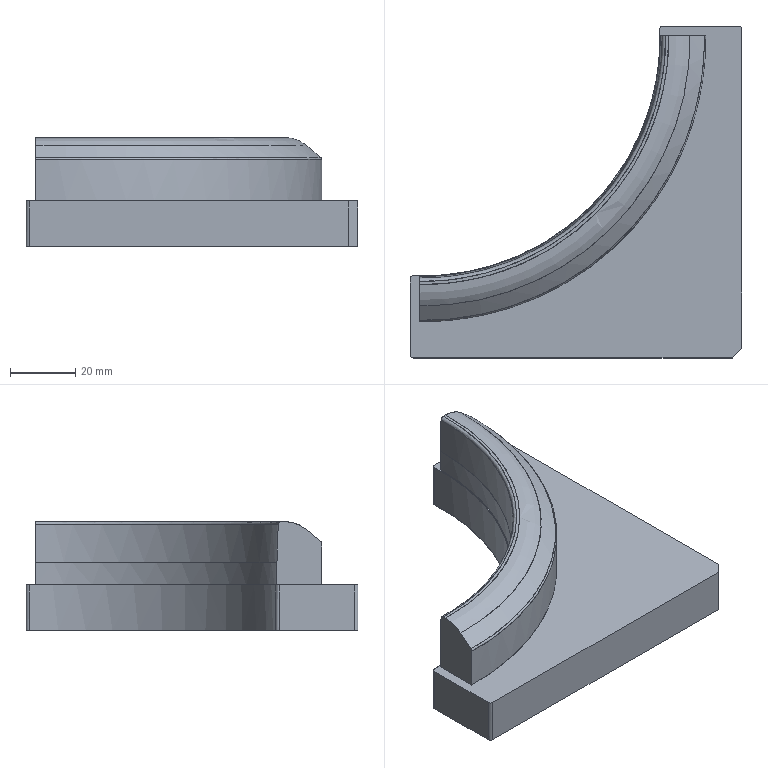NC program | PowerMill | posted with a generic post | part box 102 x 102 x 33.478 mm
Lines 26163 to 27589 of 321973:
N26260 M6
N26261 S8500 M03
N26262 G00 G90 X0.0 Y0.0
N26263 G43 Z11.798 H3
N26264
N26265 G05 P10000 R8
N26266 X-44.9733 Y-16.6515
N26267 Z0.9284
N26268 G01 Z-0.2716 F360.0
N26269 X-44.7623 Y-21.9223 F600.0
N26270 X-52.3322 Y-32.1075
N26271 X-52.0765 Y-32.4201
N26272 X-51.698 Y-32.7961
N26273 X-51.4398 Y-33.0238
N26274 X-51.2774 Y-33.1416
N26275 X-51.1104 Y-33.2689
N26276 X-50.8427 Y-33.4358
N26277 X-50.7894 Y-33.4748
N26278 X-50.4661 Y-33.6516
N26279 X-50.2251 Y-33.7596
N26280 X-50.1454 Y-33.8005
N26281 X-49.8233 Y-33.9257
N26282 X-49.497 Y-34.0292
N26283 X-49.2456 Y-34.0811
N26284 X-49.1782 Y-34.1097
N26285 X-48.8563 Y-34.167
N26286 X-48.5373 Y-34.205
N26287 X-48.2139 Y-34.2338
N26288 X-47.9403 Y-34.2383
N26289 X-38.4079 Y-21.4126
N26290 X-37.7927 Y-21.3346
N26291 X-36.8455 Y-21.201
N26292 X-36.2144 Y-21.1043
N26293 X-35.2671 Y-20.9472
N26294 X-34.636 Y-20.8355
N26295 X-33.6888 Y-20.6565
N26296 X-32.7418 Y-20.4631
N26297 X-31.5277 Y-20.1954
N26298 X-41.8701 Y-34.111
N26299 X-41.4021 Y-34.0852
N26300 X-41.2489 Y-34.0705
N26301 X-40.9258 Y-34.0486
N26302 X-40.6131 Y-34.0011
N26303 X-39.9854 Y-33.9497
N26304 X-39.3505 Y-33.912
N26305 X-38.4006 Y-33.8202
N26306 X-37.9379 Y-33.7685
N26307 X-37.7675 Y-33.7437
N26308 X-37.451 Y-33.7138
N26309 X-36.8169 Y-33.6351
N26310 X-36.5021 Y-33.5904
N26311 X-36.1825 Y-33.5538
N26312 X-35.8626 Y-33.5014
N26313 X-35.6198 Y-33.452
N26314 X-35.3807 Y-33.4197
N26315 X-23.8954 Y-17.9663
N26316 X-23.5866 Y-17.858
N26317 X-22.9558 Y-17.6264
N26318 X-21.3769 Y-17.0172
N26319 X-20.1399 Y-16.5055
N26320 X-19.4029 Y-16.1898
N26321 X-18.2203 Y-15.6594
N26322 X-16.9573 Y-15.065
N26323 X-16.0414 Y-14.6114
N26324 X-15.0494 Y-14.1042
N26325 X-28.4407 Y-32.1221
N26326 X-28.2757 Y-32.0895
N26327 X-27.9566 Y-32.0117
N26328 X-27.6359 Y-31.9409
N26329 X-27.3579 Y-31.8612
N26330 X-27.3099 Y-31.8361
N26331 X-26.6913 Y-31.6679
N26332 X-26.3741 Y-31.604
N26333 X-26.0579 Y-31.5255
N26334 X-25.4226 Y-31.3594
N26335 X-24.4741 Y-31.0918
N26336 X-23.8756 Y-30.9169
N26337 X-23.8357 Y-30.9007
N26338 X-23.209 Y-30.7123
N26339 X-22.8875 Y-30.6234
N26340 X-22.5661 Y-30.5105
N26341 X-22.3787 Y-30.4327
N26342 X-22.2613 Y-30.398
N26343 X-21.8412 Y-30.287
N26344 X-21.6225 Y-30.2161
N26345 X-21.3074 Y-30.1042
N26346 X-20.8541 Y-29.9544
N26347 X-3.3016 Y-6.3377
N26348 X-2.62 Y-5.7722
N26349 X-1.8042 Y-5.075
N26350 X-1.1729 Y-4.5225
N26351 X-0.4587 Y-3.8781
N26352 X0.0896 Y-3.3689
N26353 X0.8843 Y-2.6153
N26354 X1.8467 Y-1.6681
N26355 X2.468 Y-1.0369
N26356 X3.3707 Y-0.0897
N26357 X3.9523 Y0.5416
N26358 X4.5095 Y1.1591
N26359 X5.0782 Y1.8044
N26360 X5.6188 Y2.4358
N26361 X6.0877 Y2.9945
N26362 X6.9149 Y4.0142
N26363 X7.3505 Y4.569
N26364 X7.9821 Y5.3896
N26365 X8.3701 Y5.9082
N26366 X8.9291 Y6.6715
N26367 X9.5104 Y7.4868
N26368 X9.9448 Y8.118
N26369 X10.5075 Y8.9534
N26370 X10.9916 Y9.6965
N26371 X11.591 Y10.6435
N26372 X12.3554 Y11.9065
N26373 X12.7172 Y12.5268
N26374 X13.2609 Y13.4849
N26375 X13.6229 Y14.147
N26376 X13.98 Y14.8118
N26377 X14.4363 Y15.6945
N26378 X14.9271 Y16.6765
N26379 X15.3661 Y17.5889
N26380 X15.6599 Y18.22
N26381 X16.0871 Y19.167
N26382 X16.6704 Y20.5345
N26383 X34.2205 Y44.148
N26384 X34.246 Y44.7322
N26385 X34.269 Y45.6838
N26386 X34.2668 Y45.9989
N26387 X34.2784 Y46.9517
N26388 X34.2651 Y47.2717
N26389 X34.2403 Y47.5841
N26390 X34.2388 Y47.9011
N26391 X34.2298 Y48.218
N26392 X34.2109 Y48.5411
N26393 X34.169 Y48.8654
N26394 X34.1019 Y49.1798
N26395 X34.0826 Y49.2883
N26396 X34.0266 Y49.5072
N26397 X33.9236 Y49.8292
N26398 X33.7978 Y50.1516
N26399 X33.6465 Y50.4729
N26400 X33.465 Y50.8042
N26401 X33.4352 Y50.841
N26402 X33.3375 Y51.0
N26403 X20.7223 Y34.0264
N26404 X20.9252 Y35.1255
N26405 X21.0671 Y35.9852
N26406 X21.2025 Y36.8459
N26407 X21.4191 Y38.4243
N26408 X21.5307 Y39.3712
N26409 X21.597 Y40.0023
N26410 X21.7145 Y41.2656
N26411 X21.7648 Y41.8964
N26412 X21.8074 Y42.5278
N26413 X21.8678 Y43.6077
N26414 X29.1911 Y53.4612
N26415 X29.2555 Y53.4571
N26416 X29.5776 Y53.418
N26417 X29.8517 Y53.3677
N26418 X30.2209 Y53.2783
N26419 X30.5437 Y53.1803
N26420 X30.8973 Y53.0451
N26421 X31.1888 Y52.9092
N26422 X31.4956 Y52.7392
N26423 X31.5378 Y52.7225
N26424 X31.8298 Y52.5358
N26425 X32.023 Y52.4011
N26426 X32.1529 Y52.3001
N26427 X32.419 Y52.0775
N26428 X32.7487 Y51.7555
N26429 X33.0301 Y51.4319
N26430 X33.1176 Y51.3096
N26431 X33.2699 Y51.1099
N26432 X33.4352 Y50.841
N26433 X33.475 Y50.7891
N26434 X33.6491 Y50.4678
N26435 X33.8005 Y50.1454
N26436 X33.9257 Y49.8233
N26437 X34.0282 Y49.5015
N26438 X34.0842 Y49.2809
N26439 X34.1019 Y49.1798
N26440 X34.1704 Y48.8572
N26441 X34.2116 Y48.5341
N26442 X34.2298 Y48.218
N26443 X34.2388 Y47.9011
N26444 X34.2403 Y47.5841
N26445 X34.2653 Y47.2679
N26446 X34.2784 Y46.9464
N26447 X34.2668 Y45.9989
N26448 X34.269 Y45.6806
N26449 X34.246 Y44.7322
N26450 X34.2045 Y43.7833
N26451 X34.1998 Y43.4615
N26452 X34.146 Y42.8315
N26453 X34.1334 Y42.5193
N26454 X34.1318 Y42.2003
N26455 X34.1156 Y41.8842
N26456 X33.9998 Y40.3013
N26457 X33.884 Y39.0283
N26458 X33.834 Y38.7142
N26459 X33.7691 Y38.1527
N26460 X33.7134 Y37.4522
N26461 X33.6779 Y37.1326
N26462 X33.6317 Y36.8173
N26463 X33.4665 Y35.5506
N26464 X33.4164 Y35.2364
N26465 X33.3862 Y34.9854
N26466 X-12.3068 Y-26.4943
N26467 X-12.1313 Y-26.4169
N26468 X-11.1785 Y-25.9602
N26469 X-10.8567 Y-25.7993
N26470 X-10.5425 Y-25.6165
N26471 X-10.2304 Y-25.4527
N26472 X-9.9082 Y-25.3022
N26473 X-9.7749 Y-25.2244
N26474 X-9.594 Y-25.1569
N26475 X-9.2809 Y-24.9837
N26476 X-9.1142 Y-24.9058
N26477 X-8.5155 Y-24.5878
N26478 X-8.3296 Y-24.4801
N26479 X-8.0063 Y-24.3103
N26480 X-7.9479 Y-24.2714
N26481 X-7.6964 Y-24.1413
N26482 X-7.0646 Y-23.7841
N26483 X-6.7964 Y-23.6369
N26484 X-6.43 Y-23.401
N26485 X-6.2839 Y-23.3218
N26486 X-6.1155 Y-23.2176
N26487 X-5.7975 Y-23.0531
N26488 X-5.1705 Y-22.677
N26489 X-5.1567 Y-22.664
N26490 X-4.8483 Y-22.4913
N26491 X-4.5308 Y-22.2984
N26492 X-4.0848 Y-22.0176
N26493 X-3.627 Y-21.7347
N26494 X-3.5781 Y-21.6963
N26495 X-3.1414 Y-21.4219
N26496 X-2.6877 Y-21.1066
N26497 X-2.2098 Y-20.7927
N26498 X-2.0071 Y-20.6761
N26499 X30.7888 Y23.4504
N26500 G00 Z11.798
N26501 G05 P0
N26502 (---------------)
N26503 ( END TOOLPATH : 精公基准台01-平坦面平行-D10 )
N26504 (---------------)
N26505 ( START TOOLPATH : 精公基准台01-基准面偏置-D10 )
N26506 (---------------)
N26507 G00 X0.0 Y0.0 Z9.7984
N26508 G05 P10000 R8
N26509 X-47.5023 Y-15.0387
N26510 Z-18.48
N26511 G01 Z-19.68 F360.0
N26512 X-47.5975 Y-20.3128 F600.0
N26513 X-47.6004 Y-20.7252
N26514 G03 X-45.617 Y-20.7134 I0.5299 J77.1533
N26515 G01 X-44.4837 Y-20.6813
N26516 G03 X-42.217 Y-20.559 I-3.0409 J77.4268
N26517 G03 X-37.9216 Y-20.1168 I-4.9741 J69.4072
N26518 G03 X-34.425 Y-19.5501 I-9.5294 J69.8717
N26519 G01 X-33.7169 Y-19.4121
N26520 G03 X-29.7502 Y-18.4932 I-13.2081 J66.0374
N26521 G01 X-29.1836 Y-18.3432
N26522 G03 X-26.9169 Y-17.6816 I-20.7852 J75.4278
N26523 G03 X-22.5249 Y-16.1501 I-20.2295 J65.0766
N26524 G01 X-21.8168 Y-15.8715
N26525 X-20.6835 Y-15.4061
N26526 X-19.7784 Y-15.0168
N26527 G03 X-17.8501 Y-14.1333 I-28.5878 J64.9414
N26528 G03 X-16.1974 Y-13.3168 I-27.8477 J58.4463
N26529 G01 X-15.5835 Y-13.0008
N26530 G03 X-13.8834 Y-12.0791 I-36.156 J68.7183
N26531 G03 X-11.6168 Y-10.7499 I-34.8659 J62.052
N26532 G03 X-7.782 Y-8.2167 I-35.5326 J57.959
N26533 G01 X-7.6501 Y-8.1224
N26534 G03 X-5.3834 Y-6.4326 I-38.1634 J53.5581
N26535 G01 X-4.7716 Y-5.95
N26536 X-4.1728 Y-5.4673
N26537 X-3.3881 Y-4.8167
N26538 X-2.7218 Y-4.25
N26539 X-2.0749 Y-3.6834
N26540 G03 X-0.2269 Y-1.9833 I-51.4771 J57.8141
N26541 G01 X0.3589 Y-1.4167
N26542 X0.89 Y-0.89
N26543 X1.4167 Y-0.3589
N26544 X2.037 Y0.2833
N26545 X2.5694 Y0.85
N26546 X3.1167 Y1.4452
N26547 X3.6834 Y2.0749
N26548 X4.25 Y2.7218
N26549 G03 X5.95 Y4.7716 I-53.5505 J46.1433
N26550 G01 X6.4334 Y5.3834
N26551 G03 X7.7148 Y7.0834 I-57.1547 J44.4129
N26552 G01 X8.1214 Y7.6484
N26553 X8.5233 Y8.2167
N26554 G03 X9.9167 Y10.293 I-55.0628 J38.4589
N26555 G01 X10.3371 Y10.9525
N26556 X10.7499 Y11.6168
N26557 G03 X11.6168 Y13.0733 I-58.4313 J35.763
N26558 G03 X12.6995 Y15.0168 I-55.8056 J32.362
N26559 G01 X13.0008 Y15.5835
N26560 X13.5802 Y16.7168
N26561 G03 X14.4501 Y18.5233 I-63.9469 J31.906
N26562 G03 X15.7803 Y21.5933 I-61.0333 J28.2679
N26563 G01 X15.8715 Y21.8168
N26564 G03 X19.6287 Y34.8503 I-62.9275 J25.1989
N26565 G03 X20.0836 Y37.6836 I-68.3408 J12.4251
N26566 G01 X20.1175 Y37.9257
N26567 G03 X20.559 Y42.217 I-69.2604 J9.2932
N26568 G03 X20.7136 Y45.617 I-71.153 J4.9404
N26569 G03 X20.7228 Y47.8837 I-79.9998 J1.4556
N26570 G01 X20.7248 Y48.167
N26571 X20.741 Y48.4504
N26572 X20.7726 Y48.7337
N26573 X20.8193 Y49.017
N26574 X20.8817 Y49.3004
N26575 X20.9607 Y49.5837
N26576 X21.0566 Y49.867
N26577 X21.1707 Y50.1504
N26578 X21.2502 Y50.3239
N26579 X21.3493 Y50.5205
N26580 X21.4588 Y50.717
N26581 X21.6262 Y50.9848
N26582 X21.8406 Y51.2837
N26583 X22.0749 Y51.5671
N26584 X22.3835 Y51.8877
N26585 X22.6668 Y52.1402
N26586 X22.9615 Y52.3684
N26587 X23.2738 Y52.5767
N26588 X23.5168 Y52.7181
N26589 X23.7963 Y52.8607
N26590 X24.0835 Y52.9871
N26591 X24.3669 Y53.0928
N26592 X24.6502 Y53.1805
N26593 X24.9335 Y53.2515
N26594 X25.2169 Y53.3066
N26595 X25.5002 Y53.3464
N26596 X25.7835 Y53.3706
N26597 X26.0669 Y53.38
N26598 X39.9503 Y53.3789
N26599 X40.2336 Y53.3657
N26600 X40.517 Y53.3371
N26601 X40.8003 Y53.2932
N26602 X41.0836 Y53.2336
N26603 X41.367 Y53.1582
N26604 X41.6503 Y53.0654
N26605 X41.8636 Y52.9837
N26606 X42.217 Y52.8252
N26607 X42.5003 Y52.6746
N26608 X42.7837 Y52.5015
N26609 X42.9087 Y52.4171
N26610 X43.1295 Y52.255
N26611 X43.3503 Y52.0745
N26612 X43.5947 Y51.8504
N26613 X43.7631 Y51.6787
N26614 X43.917 Y51.507
N26615 X44.0988 Y51.2837
N26616 X44.3029 Y51.0004
N26617 X44.4837 Y50.7118
N26618 X44.6366 Y50.4311
N26619 X44.7687 Y50.1504
N26620 X44.8828 Y49.867
N26621 X44.9787 Y49.5837
N26622 X45.0503 Y49.3292
N26623 X45.1201 Y49.017
N26624 X45.1668 Y48.7337
N26625 X45.1984 Y48.4504
N26626 X45.2149 Y48.167
N26627 G02 X34.7155 Y4.25 I-92.1999 J-1.171
N26628 G02 X26.3502 Y-8.8999 I-81.6775 J42.7234
N26629 G01 X25.7873 Y-9.6312
N26630 X25.2169 Y-10.3567
N26631 X24.6502 Y-11.0628
N26632 G02 X18.9835 Y-17.4301 I-71.6609 J58.0708
N26633 G01 X18.1987 Y-18.2234
N26634 X31.7795 Y-31.8074
N26635 G02 X28.1412 Y-35.2825 I-77.9894 J78.008
N26636 G01 X27.3171 Y-36.0344
N26637 G03 X27.7283 Y-37.0998 I0.413 J-0.4527
N26638 G01 X35.7571 Y-37.1234
N26639 G03 X37.0941 Y-35.7868 I0.0039 J1.3331
N26640 G01 X37.0728 Y-27.7575
N26641 G03 X36.0076 Y-27.3461 I-0.6127 J-0.0016
N26642 G01 X35.2554 Y-28.1699
N26643 G02 X31.7795 Y-31.8074 I-81.4601 J74.3653
N26644 G01 X28.3843 Y-28.4114
N26645 G02 X14.3498 Y-40.2097 I-75.2562 J75.2741
N26646 G01 X13.4495 Y-40.8427
N26647 G03 X13.7703 Y-41.8622 I0.3225 J-0.4587
N26648 G01 X40.5758 Y-41.9435
N26649 G03 X41.9128 Y-40.6068 I0.004 J1.333
N26650 G01 X41.8392 Y-13.8045
N26651 G03 X40.8193 Y-13.4838 I-0.5608 J-0.0016
N26652 G01 X40.2524 Y-14.2915
N26653 G02 X37.7473 Y-17.7076 I-83.6931 J58.7486
N26654 G01 X37.6404 Y-17.8471
N26655 G02 X28.3843 Y-28.4114 I-84.5123 J64.7098
N26656 G01 X24.9893 Y-25.0156
N26657 G02 X-3.9856 Y-45.2937 I-71.9642 J71.9878
N26658 G01 X-4.7619 Y-45.6554
N26659 G03 X-4.5518 Y-46.6107 I0.2116 J-0.4542
N26660 G01 X45.078 Y-46.7627
N26661 G03 X45.9755 Y-46.4189 I0.004 J1.3329
N26662 G01 X46.2913 Y-46.1336
N26663 G03 X46.7308 Y-45.1408 I-0.8934 J0.9891
N26664 G01 X46.5929 Y4.5101
N26665 G03 X45.638 Y4.7213 I-0.5011 J-0.0014
N26666 G01 X45.1992 Y3.7844
N26667 G02 X33.8841 Y-14.8574 I-92.0187 J43.0981
N26668 G01 X33.87 Y-14.8758
N26669 G02 X24.9893 Y-25.0156 I-80.8445 J61.8477
N26670 G01 X21.5941 Y-21.6196
N26671 G03 X25.8575 Y-17.0746 I-68.5669 J68.5898
N26672 G01 X25.8637 Y-17.0675
N26673 G03 X42.4111 Y9.3268 I-72.8258 J64.041
N26674 G01 X42.4199 Y9.3476
N26675 G03 X50.0206 Y47.5866 I-89.341 J37.6331
N26676 G01 X50.0168 Y48.2056
N26677 X49.9788 Y48.8989
N26678 X49.7641 Y50.8652
N26679 G02 X51.0203 Y51.1091 I0.6381 J0.0705
N26680 G01 X51.2249 Y50.3794
N26681 G02 X51.27 Y50.0553 I-1.1676 J-0.3275
N26682 G01 X51.5416 Y-47.059
N26683 G02 X51.4164 Y-47.7613 I-2.0 J-0.0056
N26684 G01 X51.1701 Y-48.424
N26685 G02 X50.6359 Y-49.2116 I-1.8748 J0.6966
N26686 G01 X48.8574 Y-50.818
N26687 G02 X48.3764 Y-51.1397 I-1.3406 J1.4843
N26688 G01 X47.8717 Y-51.3799
N26689 G02 X47.006 Y-51.5741 I-0.8595 J1.8057
N26690 G01 X-50.0228 Y-51.2749
N26691 G02 X-50.3071 Y-51.2402 I0.0037 J1.2124
N26692 G01 X-51.0889 Y-51.0491
N26693 G02 X-50.8523 Y-49.7687 I0.1548 J0.6335
N26694 G01 X-48.1072 Y-50.1157
N26695 G03 X-39.5098 Y-50.0051 I3.9023 J30.8698
N26696 G01 X-32.3529 Y-48.9127
N26697 G03 X-9.6671 Y-42.5525 I-14.6218 J95.7927
N26698 G01 X-9.6345 Y-42.5389
N26699 G03 X21.5941 Y-21.6196 I-37.3404 J89.5112
N26700 G01 X18.1987 Y-18.2234
N26701 X17.2835 Y-19.1263
N26702 G02 X11.0628 Y-24.6502 I-64.2585 J66.0987
N26703 G01 X10.3567 Y-25.2169
N26704 G02 X-11.0652 Y-37.9335 I-57.3531 J72.2133
N26705 G02 X-48.167 Y-45.2145 I-35.9277 J84.906
N26706 G01 X-48.4504 Y-45.1984
N26707 X-48.7337 Y-45.1668
N26708 X-49.017 Y-45.1201
N26709 X-49.3292 Y-45.0503
N26710 X-49.5837 Y-44.9787
N26711 X-49.867 Y-44.8828
N26712 X-50.1504 Y-44.7687
N26713 X-50.4311 Y-44.6366
N26714 X-50.717 Y-44.4806
N26715 X-51.0004 Y-44.3028
N26716 X-51.2837 Y-44.0988
N26717 X-51.507 Y-43.917
N26718 X-51.6787 Y-43.7631
N26719 X-51.8504 Y-43.5947
N26720 X-52.0745 Y-43.3503
N26721 X-52.255 Y-43.1295
N26722 X-52.4171 Y-42.9087
N26723 X-52.5015 Y-42.7837
N26724 X-52.6747 Y-42.5003
N26725 X-52.8252 Y-42.217
N26726 X-52.9837 Y-41.8636
N26727 X-53.0654 Y-41.6503
N26728 X-53.158 Y-41.367
N26729 X-53.2336 Y-41.0836
N26730 X-53.2931 Y-40.8003
N26731 X-53.3371 Y-40.517
N26732 X-53.3656 Y-40.2336
N26733 X-53.3789 Y-39.9503
N26734 X-53.3801 Y-26.0669
N26735 X-53.3706 Y-25.7835
N26736 X-53.3462 Y-25.5002
N26737 X-53.3066 Y-25.2169
N26738 X-53.2515 Y-24.9335
N26739 X-53.1805 Y-24.6502
N26740 X-53.0926 Y-24.3669
N26741 X-52.9871 Y-24.0835
N26742 X-52.8608 Y-23.7963
N26743 X-52.7181 Y-23.5168
N26744 X-52.5765 Y-23.2738
N26745 X-52.4171 Y-23.0307
N26746 X-52.3601 Y-22.9502
N26747 X-52.1404 Y-22.6668
N26748 X-51.8877 Y-22.3835
N26749 X-51.7307 Y-22.2256
N26750 X-51.5671 Y-22.0745
N26751 X-51.2525 Y-21.8168
N26752 X-50.9848 Y-21.6259
N26753 X-50.717 Y-21.4588
N26754 X-50.5205 Y-21.3489
N26755 X-50.3239 Y-21.2502
N26756 X-50.1504 Y-21.1707
N26757 X-49.867 Y-21.0563
N26758 X-49.5837 Y-20.9607
N26759 X-49.3004 Y-20.8818
N26760 X-49.017 Y-20.8193
N26761 X-48.7337 Y-20.7724
N26762 X-48.4504 Y-20.741
N26763 X-48.167 Y-20.7249
N26764 X-47.6004 Y-20.7252
N26765 X-47.5975 Y-20.3128
N26766 G00 Z9.7984
N26767 G05 P0
N26768 (---------------)
N26769 ( END TOOLPATH : 精公基准台01-基准面偏置-D10 )
N26770 (---------------)
N26771 ( START TOOLPATH : 精公基准台01-外形侧光-D10 )
N26772 (---------------)
N26773 G00 X0.0 Y0.0 Z10.798
N26774 G05 P10000 R8
N26775 X19.0356 Y-17.484
N26776 Z-14.65
N26777 G01 Z-19.65 F360.0
N26778 G03 X17.9751 Y-17.9238 I0.0006 J-1.5 F600.0
N26779 G02 X13.9269 Y-21.7376 I-65.048 J64.9911
N26780 G01 X12.8309 Y-22.6934
N26781 G02 X-4.162 Y-34.2515 I-59.8408 J69.7079
N26782 G01 X-5.4409 Y-34.9132
N26783 G02 X-10.3744 Y-37.2348 I-42.0489 J82.9539
N26784 G02 X-17.5 Y-39.9867 I-36.8136 J84.7221
N26785 G02 X-35.5892 Y-44.1411 I-29.5187 J87.0706
N26786 G01 X-37.0508 Y-44.3123
N26787 G02 X-48.014 Y-44.8471 I-9.9531 J91.4064
N26788 G02 X-53.01 Y-39.7973 I0.0146 J5.0108
N26789 G01 Y-26.1041
N26790 G02 X-48.0119 Y-21.0924 I5.01 J0.0017
N26791 G03 X-37.8002 Y-20.4738 I0.9669 J68.6279
N26792 G03 X21.0965 Y46.6134 I-9.2004 J67.4739
N26793 G03 X21.0924 Y48.014 I-64.7503 J0.5105
N26794 G02 X26.1056 Y53.01 I5.0101 J-0.014
N26795 G01 X37.1235
N26796 X39.7982
N26797 G02 X44.8471 Y48.0128 I0.0383 J-5.0105
N26798 G02 X34.9127 Y5.4399 I-91.8589 J-1.0104
N26799 G01 X34.2512 Y4.1613
N26800 G02 X25.2553 Y-9.7106 I-81.2829 J42.8589
N26801 G01 X24.3692 Y-10.8215
N26802 G02 X17.9751 Y-17.9238 I-71.4416 J57.8882
N26803 G03 X17.5362 Y-18.9846 I1.0611 J-1.0602
N26804 G01 X18.979 Y-17.4274
N26805 G03 X17.9185 Y-17.8672 I0.0007 J-1.5
N26806 G02 X13.8743 Y-21.6773 I-64.9908 J64.9339
N26807 G01 X12.7789 Y-22.6325
N26808 G02 X-4.1988 Y-34.1805 I-59.7888 J69.647
N26809 G01 X-5.4767 Y-34.8417
N26810 G02 X-10.4057 Y-37.1612 I-42.0158 J82.888
N26811 G02 X-17.5254 Y-39.9108 I-36.7826 J84.6494
N26812 G02 X-35.5985 Y-44.0617 I-29.4934 J86.9953
N26813 G01 X-37.0589 Y-44.2327
N26814 G02 X-48.0123 Y-44.7671 I-9.9452 J91.3293
N26815 G02 X-52.93 Y-39.7973 I0.0129 J4.9307
N26816 G01 Y-26.1056
N26817 G02 X-48.0123 Y-21.1724 I4.93 J0.0032
N26818 G03 X-34.5031 Y-20.0233 I0.9655 J68.6338
N26819 G03 X21.1765 Y46.6127 I-12.4991 J67.0243
N26820 G03 X21.1724 Y48.0123 I-64.527 J0.5098
N26821 G02 X26.1056 Y52.93 I4.93 J-0.0123
N26822 G01 X37.1235
N26823 X39.7973
N26824 G02 X44.7671 Y48.0123 I0.0392 J-4.9304
N26825 G02 X34.8417 Y5.4767 I-91.7791 J-1.0098
N26826 G01 X34.1805 Y4.1988
N26827 G02 X25.1928 Y-9.6607 I-81.2126 J42.8217
N26828 G01 X24.3073 Y-10.7708
N26829 G02 X17.9185 Y-17.8672 I-71.3795 J57.8374
N26830 G03 X17.4797 Y-18.9281 I1.0612 J-1.0602
N26831 G00 Z10.798
N26832 G05 P0
N26833 (---------------)
N26834 ( END TOOLPATH : 精公基准台01-外形侧光-D10 )
N26835 (---------------)
N26836 ( START TOOLPATH : 精公基准台01-基准台侧光-D10 )
N26837 (---------------)
N26838 G00 X0.0 Y0.0 Z9.7984
N26839 G05 P10000 R8
N26840 X55.9652 Y-57.2901
N26841 Z-32.38
N26842 G01 Z-33.58 F360.0
N26843 G03 X52.4296 Y-53.7546 I-1.7678 J1.7677 F600.0
N26844 G01 X51.5925 Y-54.5917
N26845 X51.5919 Y-54.5923
N26846 X51.5912 Y-54.5929
N26847 X51.429 Y-54.7481
N26848 X51.4276 Y-54.7494
N26849 X51.4262 Y-54.7507
N26850 X51.2412 Y-54.9116
N26851 X51.24 Y-54.9127
N26852 X51.2387 Y-54.9137
N26853 X51.1075 Y-55.0187
N26854 X51.1058 Y-55.02
N26855 X51.1041 Y-55.0212
N26856 X50.8093 Y-55.2325
N26857 X50.8068 Y-55.2342
N26858 X50.8043 Y-55.2358
N26859 X50.4668 Y-55.4408
N26860 X50.4646 Y-55.4421
N26861 X50.4624 Y-55.4433
N26862 X50.2502 Y-55.5544
N26863 X50.2489 Y-55.5551
N26864 X50.2477 Y-55.5557
N26865 X50.1437 Y-55.6056
N26866 X50.142 Y-55.6063
N26867 X50.1403 Y-55.6071
N26868 X49.8242 Y-55.7411
N26869 X49.8217 Y-55.7422
N26870 X49.8191 Y-55.7431
N26871 X49.503 Y-55.8525
N26872 X49.5014 Y-55.8531
N26873 X49.4998 Y-55.8535
N26874 X49.424 Y-55.8763
N26875 X49.4228 Y-55.8767
N26876 X49.4215 Y-55.877
N26877 X49.1812 Y-55.9408
N26878 X49.1789 Y-55.9413
N26879 X49.1767 Y-55.9418
N26880 X48.8606 Y-56.0065
N26881 X48.858 Y-56.007
N26882 X48.8555 Y-56.0074
N26883 X48.5393 Y-56.0513
N26884 X48.5368 Y-56.0516
N26885 X48.5343 Y-56.0518
N26886 X48.2181 Y-56.0753
N26887 X48.2158 Y-56.0754
N26888 X48.2134 Y-56.0755
N26889 X47.8972 Y-56.08
N26890 X47.8966
N26891 X47.8961
N26892 X-49.7929
N26893 X-49.7931
N26894 X-49.7932
N26895 X-50.1094 Y-56.0788
N26896 X-50.111
N26897 X-50.1126 Y-56.0787
N26898 X-50.4288 Y-56.0648
N26899 X-50.4309 Y-56.0647
N26900 X-50.433 Y-56.0645
N26901 X-50.7492 Y-56.0336
N26902 X-50.7513 Y-56.0334
N26903 X-50.7534 Y-56.0331
N26904 X-51.0695 Y-55.9852
N26905 X-51.0716 Y-55.9848
N26906 X-51.0737 Y-55.9844
N26907 X-51.3899 Y-55.919
N26908 X-51.392 Y-55.9185
N26909 X-51.3941 Y-55.918
N26910 X-51.7103 Y-55.8344
N26911 X-51.7124 Y-55.8338
N26912 X-51.7145 Y-55.8332
N26913 X-52.0307 Y-55.7306
N26914 X-52.0327 Y-55.7299
N26915 X-52.0348 Y-55.7291
N26916 X-52.3509 Y-55.6071
N26917 X-52.3531 Y-55.6062
N26918 X-52.3552 Y-55.6053
N26919 X-52.6714 Y-55.4614
N26920 X-52.6735 Y-55.4604
N26921 X-52.6755 Y-55.4594
N26922 X-52.9917 Y-55.293
N26923 X-52.9938 Y-55.2918
N26924 X-52.9959 Y-55.2906
N26925 X-53.3121 Y-55.0985
N26926 X-53.314 Y-55.0973
N26927 X-53.3159 Y-55.0961
N26928 X-53.576 Y-54.9172
N26929 X-53.5781 Y-54.9156
N26930 X-53.5802 Y-54.914
N26931 X-53.9524 Y-54.6199
N26932 X-53.9548 Y-54.618
N26933 X-53.957 Y-54.616
N26934 X-54.2732 Y-54.325
N26935 X-54.2753 Y-54.3229
N26936 X-54.2774 Y-54.3208
N26937 X-54.5936 Y-53.9827
N26938 X-54.5955 Y-53.9805
N26939 X-54.5975 Y-53.9783
N26940 X-54.8722 Y-53.6368
N26941 X-54.8739 Y-53.6346
N26942 X-54.8755 Y-53.6324
N26943 X-55.0954 Y-53.3162
N26944 X-55.0968 Y-53.3142
N26945 X-55.0981 Y-53.3121
N26946 X-55.2905 Y-52.996
N26947 X-55.2918 Y-52.9939
N26948 X-55.2929 Y-52.9917
N26949 X-55.4596 Y-52.6756
N26950 X-55.4607 Y-52.6735
N26951 X-55.4617 Y-52.6713
N26952 X-55.6053 Y-52.3552
N26953 X-55.6062 Y-52.3531
N26954 X-55.6071 Y-52.351
N26955 X-55.7293 Y-52.0348
N26956 X-55.7301 Y-52.0327
N26957 X-55.7308 Y-52.0306
N26958 X-55.8332 Y-51.7145
N26959 X-55.8339 Y-51.7124
N26960 X-55.8345 Y-51.7102
N26961 X-55.918 Y-51.3941
N26962 X-55.9185 Y-51.3919
N26963 X-55.919 Y-51.3897
N26964 X-55.9838 Y-51.0736
N26965 X-55.9842 Y-51.0716
N26966 X-55.9845 Y-51.0697
N26967 X-56.0331 Y-50.7535
N26968 X-56.0334 Y-50.7513
N26969 X-56.0336 Y-50.749
N26970 X-56.0639 Y-50.4329
N26971 X-56.0641 Y-50.4309
N26972 X-56.0642 Y-50.4289
N26973 X-56.0787 Y-50.1128
N26974 X-56.0788 Y-50.1111
N26975 Y-50.1094
N26976 X-56.08 Y-49.7932
N26977 Y-49.7931
N26978 Y-49.7929
N26979 Y-26.7143
N26980 X-56.0799 Y-26.7131
N26981 Y-26.7119
N26982 X-56.0704 Y-26.3957
N26983 X-56.0703 Y-26.3937
N26984 X-56.0701 Y-26.3916
N26985 X-56.044 Y-26.0754
N26986 X-56.0438 Y-26.0733
N26987 X-56.0435 Y-26.0712
N26988 X-56.0003 Y-25.755
N26989 X-56.0 Y-25.7529
N26990 X-55.9996 Y-25.7508
N26991 X-55.939 Y-25.4347
N26992 X-55.9387 Y-25.4328
N26993 X-55.9382 Y-25.4309
N26994 X-55.8775 Y-25.1802
N26995 X-55.8769 Y-25.1781
N26996 X-55.8763 Y-25.176
N26997 X-55.7615 Y-24.7944
N26998 X-55.7608 Y-24.792
N26999 X-55.76 Y-24.7897
N27000 X-55.643 Y-24.4735
N27001 X-55.6422 Y-24.4715
N27002 X-55.6413 Y-24.4694
N27003 X-55.504 Y-24.1533
N27004 X-55.503 Y-24.151
N27005 X-55.5019 Y-24.1488
N27006 X-55.341 Y-23.8327
N27007 X-55.3402 Y-23.8313
N27008 X-55.3394 Y-23.8298
N27009 X-55.2372 Y-23.6478
N27010 X-55.2365 Y-23.6465
N27011 X-55.2357 Y-23.6453
N27012 X-55.154 Y-23.5112
N27013 X-55.1531 Y-23.5098
N27014 X-55.1521 Y-23.5083
N27015 X-54.9402 Y-23.1922
N27016 X-54.9387 Y-23.19
N27017 X-54.9372 Y-23.1879
N27018 X-54.6939 Y-22.8718
N27019 X-54.6927 Y-22.8703
N27020 X-54.6916 Y-22.8689
N27021 X-54.5962 Y-22.7561
N27022 X-54.5953 Y-22.755
N27023 X-54.5944 Y-22.754
N27024 X-54.4099 Y-22.5507
N27025 X-54.4089 Y-22.5495
N27026 X-54.4078 Y-22.5484
N27027 X-54.2761 Y-22.4141
N27028 X-54.2751 Y-22.4131
N27029 X-54.274 Y-22.412
N27030 X-54.0819 Y-22.2302
N27031 X-54.0809 Y-22.2292
N27032 X-54.0798 Y-22.2282
N27033 X-53.9557 Y-22.119
N27034 X-53.9545 Y-22.1179
N27035 X-53.9532 Y-22.1168
N27036 X-53.6978 Y-21.91
N27037 X-53.6957 Y-21.9083
N27038 X-53.6936 Y-21.9068
N27039 X-53.3167 Y-21.6406
N27040 X-53.3144 Y-21.639
N27041 X-53.312 Y-21.6375
N27042 X-52.9959 Y-21.4458
N27043 X-52.9938 Y-21.4446
N27044 X-52.9917 Y-21.4434
N27045 X-52.6755 Y-21.277
N27046 X-52.6735 Y-21.2759
N27047 X-52.6714 Y-21.275
N27048 X-52.3553 Y-21.1309
N27049 X-52.3531 Y-21.13
N27050 X-52.351 Y-21.1291
N27051 X-52.0348 Y-21.0068
N27052 X-52.0327 Y-21.006
N27053 X-52.0306 Y-21.0053
N27054 X-51.7145 Y-20.9029
N27055 X-51.7124 Y-20.9023
N27056 X-51.7102 Y-20.9017
N27057 X-51.3941 Y-20.8182
N27058 X-51.392 Y-20.8177
N27059 X-51.3899 Y-20.8172
N27060 X-51.0737 Y-20.7518
N27061 X-51.0716 Y-20.7513
N27062 X-51.0694 Y-20.751
N27063 X-50.7532 Y-20.7036
N27064 X-50.7513 Y-20.7033
N27065 X-50.7493 Y-20.7031
N27066 X-50.4332 Y-20.6716
N27067 X-50.4308 Y-20.6714
N27068 X-50.4285 Y-20.6713
N27069 X-50.1123 Y-20.6586
N27070 X-50.1105 Y-20.6585
N27071 X-50.1088
N27072 X-49.7926 Y-20.6598
N27073 X-49.7915
N27074 X-49.7904
N27075 X-48.8425 Y-20.6905
N27076 X-47.5792 Y-20.7131
N27077 X-46.632 Y-20.7144
N27078 X-45.3688 Y-20.6959
N27079 X-44.1056 Y-20.6539
N27080 X-43.1585 Y-20.6066
N27081 X-41.8952 Y-20.5229
N27082 X-40.9481 Y-20.4447
N27083 X-39.6848 Y-20.3191
N27084 X-38.7377 Y-20.2094
N27085 X-37.4744 Y-20.0426
N27086 X-36.5273 Y-19.9011
N27087 X-35.264 Y-19.691
N27088 X-34.3169 Y-19.5174
N27089 X-33.0537 Y-19.2636
N27090 X-31.7905 Y-18.9855
N27091 X-30.8433 Y-18.7601
N27092 X-29.8961 Y-18.5199
N27093 X-28.6328 Y-18.1772
N27094 X-27.6856 Y-17.9028
N27095 X-26.7381 Y-17.6132
N27096 X-26.2886 Y-17.47
N27097 X-25.3285 Y-17.1541
N27098 X-24.415 Y-16.8384
N27099 X-23.2647 Y-16.4199
N27100 X-22.3175 Y-16.0572
N27101 X-21.1213 Y-15.5753
N27102 X-20.107 Y-15.146
N27103 X-19.1597 Y-14.7274
N27104 X-18.2567 Y-14.3122
N27105 X-17.265 Y-13.8377
N27106 X-16.3177 Y-13.3657
N27107 X-15.3704 Y-12.8751
N27108 X-14.4231 Y-12.3647
N27109 X-13.4758 Y-11.8347
N27110 X-12.5285 Y-11.2846
N27111 X-11.5812 Y-10.7138
N27112 X-10.6338 Y-10.1215
N27113 X-9.6865 Y-9.5074
N27114 X-8.7392 Y-8.8705
N27115 X-7.7919 Y-8.21
N27116 X-6.8446 Y-7.5248
N27117 X-5.8973 Y-6.8139
N27118 X-4.9812 Y-6.1021
N27119 X-4.1949 Y-5.4706
N27120 X-3.3711 Y-4.7875
N27121 X-2.4238 Y-3.9741
N27122 X-1.4764 Y-3.1296
N27123 X-0.5923 Y-2.3128
N27124 X0.07 Y-1.6813
N27125 X0.3926 Y-1.3657
N27126 X1.0299 Y-0.7339
N27127 X1.6498 Y-0.1024
N27128 X2.3128 Y0.5923
N27129 X3.1296 Y1.4764
N27130 X3.8917 Y2.3298
N27131 X4.5232 Y3.0597
N27132 X5.3135 Y4.0026
N27133 X6.0775 Y4.95
N27134 X6.7336 Y5.7922
N27135 X7.5249 Y6.8447
N27136 X7.9838 Y7.476
N27137 X8.6283 Y8.3879
N27138 X9.2598 Y9.314
N27139 X9.8914 Y10.2743
N27140 X10.5191 Y11.2654
N27141 X11.0966 Y12.2127
N27142 X11.6534 Y13.16
N27143 X12.19 Y14.1074
N27144 X12.7067 Y15.0547
N27145 X13.2037 Y16.002
N27146 X13.6807 Y16.947
N27147 X13.9903 Y17.5808
N27148 X14.4386 Y18.5282
N27149 X14.8692 Y19.4755
N27150 X15.2595 Y20.3697
N27151 X15.6778 Y21.3701
N27152 X16.0571 Y22.3174
N27153 X16.4199 Y23.2647
N27154 X16.7658 Y24.2121
N27155 X16.9874 Y24.8435
N27156 X17.3081 Y25.791
N27157 X17.6133 Y26.7383
N27158 X17.9028 Y27.6856
N27159 X18.1773 Y28.6329
N27160 X18.4365 Y29.5801
N27161 X18.7601 Y30.8434
N27162 X18.9855 Y31.7905
N27163 X19.2636 Y33.0537
N27164 X19.5174 Y34.3169
N27165 X19.691 Y35.2641
N27166 X19.8508 Y36.2113
N27167 X20.0426 Y37.4746
N27168 X20.1702 Y38.4217
N27169 X20.3119 Y39.617
N27170 X20.4154 Y40.6322
N27171 X20.5229 Y41.8954
N27172 X20.5879 Y42.8426
N27173 X20.6539 Y44.1058
N27174 X20.6875 Y45.053
N27175 X20.7121 Y46.3162
N27176 X20.7149 Y47.2634
N27177 X20.6983 Y48.531
N27178 X20.6598 Y49.7905
N27179 Y49.7914
N27180 Y49.7923
N27181 X20.6572 Y50.1084
N27182 Y50.1105
N27183 X20.6573 Y50.1126
N27184 X20.6713 Y50.4288
N27185 X20.6715 Y50.4309
N27186 X20.6716 Y50.433
N27187 X20.7025 Y50.7492
N27188 X20.7028 Y50.7513
N27189 X20.703 Y50.7534
N27190 X20.751 Y51.0695
N27191 X20.7514 Y51.0716
N27192 X20.7518 Y51.0737
N27193 X20.8172 Y51.3899
N27194 X20.8177 Y51.392
N27195 X20.8182 Y51.3941
N27196 X20.9017 Y51.7102
N27197 X20.9023 Y51.7124
N27198 X20.9029 Y51.7145
N27199 X21.0053 Y52.0306
N27200 X21.006 Y52.0327
N27201 X21.0068 Y52.0348
N27202 X21.1291 Y52.351
N27203 X21.13 Y52.3531
N27204 X21.1309 Y52.3552
N27205 X21.267 Y52.6552
N27206 X21.268 Y52.6573
N27207 X21.269 Y52.6593
N27208 X21.4433 Y52.9916
N27209 X21.4445 Y52.9938
N27210 X21.4458 Y52.9959
N27211 X21.6376 Y53.312
N27212 X21.6389 Y53.3142
N27213 X21.6403 Y53.3163
N27214 X21.8606 Y53.6324
N27215 X21.8622 Y53.6346
N27216 X21.8638 Y53.6366
N27217 X22.1165 Y53.9528
N27218 X22.1177 Y53.9543
N27219 X22.119 Y53.9557
N27220 X22.2282 Y54.0798
N27221 X22.2292 Y54.0809
N27222 X22.2302 Y54.0819
N27223 X22.412 Y54.274
N27224 X22.4131 Y54.2751
N27225 X22.4141 Y54.2761
N27226 X22.5484 Y54.4078
N27227 X22.5495 Y54.4089
N27228 X22.5507 Y54.4099
N27229 X22.754 Y54.5944
N27230 X22.755 Y54.5953
N27231 X22.7561 Y54.5962
N27232 X22.8689 Y54.6916
N27233 X22.8702 Y54.6927
N27234 X22.8716 Y54.6937
N27235 X23.1566 Y54.9145
N27236 X23.1587 Y54.9161
N27237 X23.1608 Y54.9176
N27238 X23.5081 Y55.152
N27239 X23.5096 Y55.153
N27240 X23.5112 Y55.154
N27241 X23.6453 Y55.2357
N27242 X23.6465 Y55.2365
N27243 X23.6478 Y55.2372
N27244 X23.8298 Y55.3394
N27245 X23.8313 Y55.3402
N27246 X23.8327 Y55.341
N27247 X24.1488 Y55.5019
N27248 X24.151 Y55.503
N27249 X24.1533 Y55.504
N27250 X24.4694 Y55.6413
N27251 X24.4715 Y55.6422
N27252 X24.4735 Y55.643
N27253 X24.7897 Y55.76
N27254 X24.7918 Y55.7607
N27255 X24.7939 Y55.7614
N27256 X25.1101 Y55.8585
N27257 X25.1122 Y55.8591
N27258 X25.1143 Y55.8597
N27259 X25.4305 Y55.9381
N27260 X25.4326 Y55.9386
N27261 X25.4347 Y55.939
N27262 X25.7508 Y55.9996
N27263 X25.7529 Y56.0
N27264 X25.755 Y56.0003
N27265 X26.0712 Y56.0435
N27266 X26.0733 Y56.0438
N27267 X26.0754 Y56.044
N27268 X26.3916 Y56.0701
N27269 X26.3937 Y56.0703
N27270 X26.3958 Y56.0704
N27271 X26.7119 Y56.0799
N27272 X26.7131
N27273 X26.7143 Y56.08
N27274 X49.7929
N27275 X49.7931
N27276 X49.7932
N27277 X50.1094 Y56.0788
N27278 X50.111
N27279 X50.1126 Y56.0787
N27280 X50.4288 Y56.0648
N27281 X50.4309 Y56.0647
N27282 X50.433 Y56.0645
N27283 X50.7492 Y56.0336
N27284 X50.7513 Y56.0334
N27285 X50.7534 Y56.0331
N27286 X51.0695 Y55.9852
N27287 X51.0716 Y55.9848
N27288 X51.0737 Y55.9844
N27289 X51.3899 Y55.919
N27290 X51.392 Y55.9185
N27291 X51.3941 Y55.918
N27292 X51.7103 Y55.8344
N27293 X51.7124 Y55.8338
N27294 X51.7145 Y55.8332
N27295 X52.0307 Y55.7306
N27296 X52.0327 Y55.7299
N27297 X52.0348 Y55.7291
N27298 X52.3509 Y55.6071
N27299 X52.3531 Y55.6062
N27300 X52.3552 Y55.6053
N27301 X52.6714 Y55.4614
N27302 X52.6735 Y55.4604
N27303 X52.6755 Y55.4594
N27304 X52.9917 Y55.293
N27305 X52.9938 Y55.2918
N27306 X52.9959 Y55.2906
N27307 X53.3121 Y55.0985
N27308 X53.314 Y55.0973
N27309 X53.3159 Y55.0961
N27310 X53.576 Y54.9172
N27311 X53.5781 Y54.9156
N27312 X53.5802 Y54.914
N27313 X53.9524 Y54.6199
N27314 X53.9548 Y54.618
N27315 X53.957 Y54.616
N27316 X54.2732 Y54.325
N27317 X54.2753 Y54.3229
N27318 X54.2774 Y54.3208
N27319 X54.5936 Y53.9827
N27320 X54.5955 Y53.9805
N27321 X54.5975 Y53.9783
N27322 X54.8722 Y53.6368
N27323 X54.8739 Y53.6346
N27324 X54.8755 Y53.6324
N27325 X55.0954 Y53.3162
N27326 X55.0968 Y53.3142
N27327 X55.0981 Y53.3121
N27328 X55.2905 Y52.996
N27329 X55.2918 Y52.9939
N27330 X55.2929 Y52.9917
N27331 X55.4596 Y52.6756
N27332 X55.4607 Y52.6735
N27333 X55.4617 Y52.6713
N27334 X55.6053 Y52.3552
N27335 X55.6062 Y52.3531
N27336 X55.607 Y52.351
N27337 X55.7293 Y52.0348
N27338 X55.7301 Y52.0327
N27339 X55.7308 Y52.0306
N27340 X55.8332 Y51.7145
N27341 X55.8339 Y51.7124
N27342 X55.8345 Y51.7102
N27343 X55.918 Y51.3941
N27344 X55.9185 Y51.3919
N27345 X55.919 Y51.3897
N27346 X55.9838 Y51.0736
N27347 X55.9842 Y51.0716
N27348 X55.9845 Y51.0697
N27349 X56.0331 Y50.7535
N27350 X56.0334 Y50.7513
N27351 X56.0336 Y50.749
N27352 X56.0639 Y50.4329
N27353 X56.0641 Y50.4309
N27354 X56.0642 Y50.4289
N27355 X56.0787 Y50.1128
N27356 X56.0788 Y50.1111
N27357 Y50.1094
N27358 X56.08 Y49.7932
N27359 Y49.7931
N27360 Y49.7929
N27361 Y0.9484
N27362 Y-47.8961
N27363 Y-47.8966
N27364 Y-47.8972
N27365 X56.0755 Y-48.2134
N27366 X56.0754 Y-48.2158
N27367 X56.0753 Y-48.2181
N27368 X56.0518 Y-48.5343
N27369 X56.0516 Y-48.5368
N27370 X56.0513 Y-48.5393
N27371 X56.0074 Y-48.8555
N27372 X56.007 Y-48.858
N27373 X56.0065 Y-48.8606
N27374 X55.9418 Y-49.1767
N27375 X55.9412 Y-49.1792
N27376 X55.9406 Y-49.1818
N27377 X55.8541 Y-49.4979
N27378 X55.8534 Y-49.5005
N27379 X55.8525 Y-49.503
N27380 X55.7431 Y-49.8191
N27381 X55.7422 Y-49.8217
N27382 X55.7411 Y-49.8242
N27383 X55.6071 Y-50.1403
N27384 X55.6063 Y-50.142
N27385 X55.6056 Y-50.1437
N27386 X55.5557 Y-50.2477
N27387 X55.5551 Y-50.2489
N27388 X55.5544 Y-50.2502
N27389 X55.4433 Y-50.4624
N27390 X55.4422 Y-50.4645
N27391 X55.4409 Y-50.4666
N27392 X55.25 Y-50.7827
N27393 X55.2484 Y-50.7853
N27394 X55.2466 Y-50.7878
N27395 X55.0214 Y-51.104
N27396 X55.0201 Y-51.1057
N27397 X55.0187 Y-51.1075
N27398 X54.9137 Y-51.2387
N27399 X54.9127 Y-51.24
N27400 X54.9116 Y-51.2412
N27401 X54.7507 Y-51.4262
N27402 X54.7494 Y-51.4276
N27403 X54.7481 Y-51.429
N27404 X54.5929 Y-51.5912
N27405 X54.5923 Y-51.5919
N27406 X54.5917 Y-51.5925
N27407 X52.4296 Y-53.7546
N27408 G03 X55.9652 Y-57.2901 I1.7678 J-1.7678
N27409 G01 X55.9137 Y-57.2285
N27410 G03 X52.3781 Y-53.693 I-1.7678 J1.7678
N27411 G01 X51.536 Y-54.5351
N27412 X51.3737 Y-54.6903
N27413 X51.1887 Y-54.8513
N27414 X51.0575 Y-54.9562
N27415 X50.7627 Y-55.1674
N27416 X50.4252 Y-55.3725
N27417 X50.2131 Y-55.4836
N27418 X50.1091 Y-55.5334
N27419 X49.7929 Y-55.6675
N27420 X49.4768 Y-55.7769
N27421 X49.401 Y-55.7997
N27422 X49.1607 Y-55.8634
N27423 X48.8445 Y-55.9282
N27424 X48.5284 Y-55.972
N27425 X48.2122 Y-55.9955
N27426 X47.8961 Y-56.0
N27427 X-49.7929
N27428 X-50.1091 Y-55.9988
N27429 X-50.4252 Y-55.9849
N27430 X-50.7414 Y-55.954
N27431 X-51.0575 Y-55.9061
N27432 X-51.3737 Y-55.8406
N27433 X-51.6898 Y-55.7571
N27434 X-52.006 Y-55.6545
N27435 X-52.3221 Y-55.5324
N27436 X-52.6383 Y-55.3886
N27437 X-52.9544 Y-55.2222
N27438 X-53.2705 Y-55.0302
N27439 X-53.5306 Y-54.8513
N27440 X-53.9028 Y-54.5571
N27441 X-54.219 Y-54.2661
N27442 X-54.5351 Y-53.9281
N27443 X-54.8099 Y-53.5867
N27444 X-55.0298 Y-53.2705
N27445 X-55.2222 Y-52.9544
N27446 X-55.3889 Y-52.6383
N27447 X-55.5324 Y-52.3221
N27448 X-55.6547 Y-52.006
N27449 X-55.7571 Y-51.6898
N27450 X-55.8406 Y-51.3737
N27451 X-55.9054 Y-51.0575
N27452 X-55.954 Y-50.7414
N27453 X-55.9843 Y-50.4252
N27454 X-55.9988 Y-50.1091
N27455 X-56.0 Y-49.7929
N27456 Y-26.7143
N27457 X-55.9904 Y-26.3982
N27458 X-55.9642 Y-26.082
N27459 X-55.921 Y-25.7659
N27460 X-55.8605 Y-25.4497
N27461 X-55.7997 Y-25.199
N27462 X-55.6849 Y-24.8174
N27463 X-55.568 Y-24.5013
N27464 X-55.4306 Y-24.1851
N27465 X-55.2697 Y-23.869
N27466 X-55.1674 Y-23.6869
N27467 X-55.0857 Y-23.5529
N27468 X-54.8738 Y-23.2367
N27469 X-54.6305 Y-22.9206
N27470 X-54.5351 Y-22.8077
N27471 X-54.3507 Y-22.6044
N27472 X-54.219 Y-22.4701
N27473 X-54.0269 Y-22.2883
N27474 X-53.9028 Y-22.179
N27475 X-53.6475 Y-21.9721
N27476 X-53.2705 Y-21.7059
N27477 X-52.9544 Y-21.5142
N27478 X-52.6383 Y-21.3478
N27479 X-52.3221 Y-21.2037
N27480 X-52.006 Y-21.0814
N27481 X-51.6898 Y-20.979
N27482 X-51.3737 Y-20.8955
N27483 X-51.0575 Y-20.8301
N27484 X-50.7414 Y-20.7827
N27485 X-50.4252 Y-20.7512
N27486 X-50.1091 Y-20.7385
N27487 X-49.7929 Y-20.7398
N27488 X-48.8445 Y-20.7705
N27489 X-47.5799 Y-20.7931
N27490 X-46.6315 Y-20.7944
N27491 X-45.3669 Y-20.7758
N27492 X-44.1023 Y-20.7338
N27493 X-43.1539 Y-20.6865
N27494 X-41.8893 Y-20.6027
N27495 X-40.9409 Y-20.5243
N27496 X-39.6763 Y-20.3987
N27497 X-38.7278 Y-20.2888
N27498 X-37.4633 Y-20.1218
N27499 X-36.5148 Y-19.9802
N27500 X-35.2502 Y-19.7698
N27501 X-34.3018 Y-19.5959
N27502 X-33.0372 Y-19.3419
N27503 X-31.7726 Y-19.0635
N27504 X-30.8242 Y-18.8378
N27505 X-29.8758 Y-18.5973
N27506 X-28.6112 Y-18.2543
N27507 X-27.6627 Y-17.9795
N27508 X-26.7143 Y-17.6896
N27509 X-26.2639 Y-17.5461
N27510 X-25.3029 Y-17.2299
N27511 X-24.3882 Y-16.9138
N27512 X-23.2367 Y-16.4948
N27513 X-22.2883 Y-16.1316
N27514 X-21.0907 Y-15.6492
N27515 X-20.0753 Y-15.2194
N27516 X-19.1268 Y-14.8004
N27517 X-18.2227 Y-14.3846
N27518 X-17.2299 Y-13.9096
N27519 X-16.2815 Y-13.437
N27520 X-15.3331 Y-12.9458
N27521 X-14.3846 Y-12.4348
N27522 X-13.4362 Y-11.9042
N27523 X-12.4878 Y-11.3535
N27524 X-11.5393 Y-10.782
N27525 X-10.5909 Y-10.189
N27526 X-9.6424 Y-9.5742
N27527 X-8.694 Y-8.9365
N27528 X-7.7456 Y-8.2752
N27529 X-6.7971 Y-7.5893
N27530 X-5.8487 Y-6.8774
N27531 X-4.9316 Y-6.1648
N27532 X-4.1444 Y-5.5325
N27533 X-3.3195 Y-4.8486
N27534 X-2.3711 Y-4.0343
N27535 X-1.4227 Y-3.1889
N27536 X-0.5376 Y-2.3711
N27537 X0.1256 Y-1.7388
N27538 X0.4487 Y-1.4227
N27539 X1.0866 Y-0.7904
N27540 X1.7072 Y-0.1581
N27541 X2.3711 Y0.5376
N27542 X3.1889 Y1.4227
N27543 X3.9518 Y2.277
N27544 X4.5841 Y3.0078
N27545 X5.3753 Y3.9518
N27546 X6.1402 Y4.9003
N27547 X6.7971 Y5.7435
N27548 X7.5892 Y6.7971
N27549 X8.0489 Y7.4294
N27550 X8.694 Y8.3423
N27551 X9.3263 Y9.2695
N27552 X9.9586 Y10.231
N27553 X10.5871 Y11.2232
N27554 X11.1652 Y12.1716
N27555 X11.7226 Y13.12
N27556 X12.2599 Y14.0685
N27557 X12.7772 Y15.0169
N27558 X13.2748 Y15.9654
N27559 X13.7523 Y16.9114
N27560 X14.0624 Y17.5461
N27561 X14.5111 Y18.4945
N27562 X14.9422 Y19.443
N27563 X15.3331 Y20.3382
N27564 X15.7519 Y21.3398
N27565 X16.1316 Y22.2883
N27566 X16.4948 Y23.2367
N27567 X16.8411 Y24.1851
N27568 X17.0631 Y24.8174
N27569 X17.384 Y25.7659
N27570 X17.6896 Y26.7143
N27571 X17.9795 Y27.6627
N27572 X18.2543 Y28.6112
N27573 X18.5138 Y29.5596
N27574 X18.8378 Y30.8242
N27575 X19.0635 Y31.7726
N27576 X19.3419 Y33.0372
N27577 X19.5959 Y34.3018
N27578 X19.7698 Y35.2502
N27579 X19.9298 Y36.1987
N27580 X20.1218 Y37.4633
N27581 X20.2496 Y38.4117
N27582 X20.3914 Y39.6082
N27583 X20.495 Y40.6247
N27584 X20.6027 Y41.8893
N27585 X20.6677 Y42.8377
N27586 X20.7338 Y44.1023
N27587 X20.7675 Y45.0508
N27588 X20.7921 Y46.3153
N27589 X20.7949 Y47.2638
N27590 X20.7784 Y48.5284
N27591 X20.7783 Y48.5327
N27592 X20.7398 Y49.7929
N27593 X20.7372 Y50.1091
N27594 X20.7513 Y50.4252
N27595 X20.7821 Y50.7414
N27596 X20.8301 Y51.0575
N27597 X20.8955 Y51.3737
N27598 X20.979 Y51.6898
N27599 X21.0814 Y52.006
N27600 X21.2037 Y52.3221
N27601 X21.3398 Y52.6222
N27602 X21.5142 Y52.9544
N27603 X21.706 Y53.2705
N27604 X21.9263 Y53.5867
N27605 X22.179 Y53.9028
N27606 X22.2883 Y54.0269
N27607 X22.4701 Y54.219
N27608 X22.6044 Y54.3507
N27609 X22.8077 Y54.5351
N27610 X22.9206 Y54.6305
N27611 X23.2056 Y54.8513
N27612 X23.5529 Y55.0857
N27613 X23.6869 Y55.1674
N27614 X23.869 Y55.2697
N27615 X24.1851 Y55.4306
N27616 X24.5013 Y55.568
N27617 X24.8174 Y55.6849
N27618 X25.1336 Y55.782
N27619 X25.4497 Y55.8605
N27620 X25.7659 Y55.921
N27621 X26.082 Y55.9642
N27622 X26.3982 Y55.9904
N27623 X26.7143 Y56.0
N27624 X49.7929
N27625 X50.1091 Y55.9988
N27626 X50.4252 Y55.9849
N27627 X50.7414 Y55.954
N27628 X51.0575 Y55.9061
N27629 X51.3737 Y55.8406
N27630 X51.6898 Y55.7571
N27631 X52.006 Y55.6545
N27632 X52.3221 Y55.5324
N27633 X52.6383 Y55.3886
N27634 X52.9544 Y55.2222
N27635 X53.2705 Y55.0302
N27636 X53.5306 Y54.8513
N27637 X53.9028 Y54.5571
N27638 X54.219 Y54.2661
N27639 X54.5351 Y53.9281
N27640 X54.8099 Y53.5867
N27641 X55.0298 Y53.2705
N27642 X55.2222 Y52.9544
N27643 X55.3888 Y52.6383
N27644 X55.5324 Y52.3221
N27645 X55.6547 Y52.006
N27646 X55.7571 Y51.6898
N27647 X55.8406 Y51.3737
N27648 X55.9055 Y51.0575
N27649 X55.954 Y50.7414
N27650 X55.9843 Y50.4252
N27651 X55.9988 Y50.1091
N27652 X56.0 Y49.7929
N27653 Y0.9484
N27654 Y-47.8961
N27655 X55.9955 Y-48.2122
N27656 X55.972 Y-48.5284
N27657 X55.9282 Y-48.8445
N27658 X55.8634 Y-49.1607
N27659 X55.7769 Y-49.4768
N27660 X55.6675 Y-49.7929
N27661 X55.5334 Y-50.1091
N27662 X55.4836 Y-50.2131
N27663 X55.3725 Y-50.4252
N27664 X55.1815 Y-50.7414
N27665 X54.9562 Y-51.0575
N27666 X54.8513 Y-51.1887
N27667 X54.6903 Y-51.3737
N27668 X54.5351 Y-51.536
N27669 X52.3781 Y-53.693
N27670 G03 X55.9137 Y-57.2285 I1.7678 J-1.7677
N27671 G00 Z9.7984
N27672 G05 P0
N27673 (---------------)
N27674 ( END TOOLPATH : 精公基准台01-基准台侧光-D10 )
N27675 (---------------)
N27676
N27677 M05
N27678 G53 Z0.0
N27679 (---------------)
N27680 ( START TOOLPATH : 精公精光01-平行-R2 )
N27681 (---------------)
N27682 ( TOOL NO.    :7 )
N27683 ( TOOL TYPE   : BALLNOSED)
N27684 ( TOOL ID     : R2_1_1_1)
N27685 ( TOOL DIA    : 4.0 LENGTH 69.84)
N27686 T7